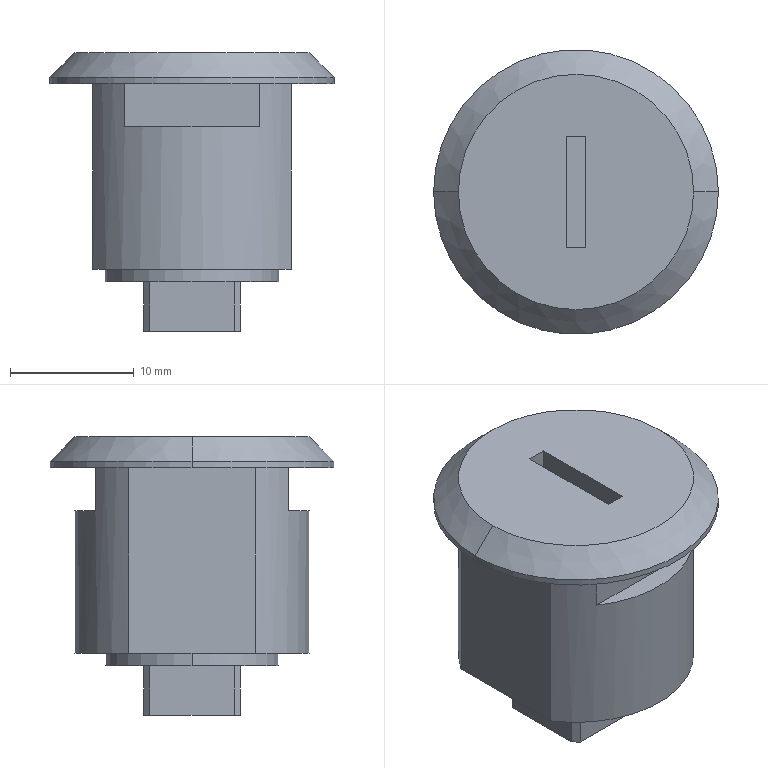Part | SolidWorks | features BaseBody 1 | 1 solid | 35 faces | box 23 x 23 x 22.5 mm | volume 4876 mm3 | plane 25 | cylinder 8 | cone 2 | commonest cylinder face diameters 3.545 x2 14 x2 19 x2 23 x2
STEP:
#1=CARTESIAN_POINT('',(9.6,1003.,461.7));
#2=VERTEX_POINT('',#1);
#3=CARTESIAN_POINT('',(-9.4,1003.,461.7));
#4=VERTEX_POINT('',#3);
#5=CARTESIAN_POINT('',(0.1,1003.,461.7));
#6=DIRECTION('',(0.,0.,-1.));
#7=DIRECTION('',(1.,0.,0.));
#8=AXIS2_PLACEMENT_3D('',#5,#6,#7);
#9=CIRCLE('',#8,9.5);
#10=EDGE_CURVE('',#2,#4,#9,.T.);
#11=ORIENTED_EDGE('',*,*,#10,.T.);
#12=CARTESIAN_POINT('',(-11.4,1003.,459.7));
#13=VERTEX_POINT('',#12);
#14=CARTESIAN_POINT('',(-11.4,1003.,459.7));
#15=DIRECTION('',(-0.7071,0.,-0.7071));
#16=VECTOR('',#15,1000.);
#17=LINE('',#14,#16);
#18=EDGE_CURVE('',#4,#13,#17,.T.);
#19=ORIENTED_EDGE('',*,*,#18,.T.);
#20=CARTESIAN_POINT('',(11.6,1003.,459.7));
#21=VERTEX_POINT('',#20);
#22=CARTESIAN_POINT('',(0.1,1003.,459.7));
#23=DIRECTION('',(0.,0.,1.));
#24=DIRECTION('',(1.,0.,0.));
#25=AXIS2_PLACEMENT_3D('',#22,#23,#24);
#26=CIRCLE('',#25,11.5);
#27=EDGE_CURVE('',#13,#21,#26,.T.);
#28=ORIENTED_EDGE('',*,*,#27,.T.);
#29=CARTESIAN_POINT('',(11.6,1003.,459.7));
#30=DIRECTION('',(0.7071,0.,-0.7071));
#31=VECTOR('',#30,1000.);
#32=LINE('',#29,#31);
#33=EDGE_CURVE('',#2,#21,#32,.T.);
#34=ORIENTED_EDGE('',*,*,#33,.F.);
#35=EDGE_LOOP('',(#11,#19,#28,#34));
#36=FACE_OUTER_BOUND('',#35,.T.);
#37=CARTESIAN_POINT('',(0.1,1003.,459.7));
#38=DIRECTION('',(0.,0.,-1.));
#39=DIRECTION('',(1.,0.,0.));
#40=AXIS2_PLACEMENT_3D('',#37,#38,#39);
#41=CONICAL_SURFACE('',#40,11.5,0.7854);
#42=ADVANCED_FACE('',(#36),#41,.T.);
#43=ORIENTED_EDGE('',*,*,#27,.F.);
#44=CARTESIAN_POINT('',(-11.4,1003.,459.2));
#45=VERTEX_POINT('',#44);
#46=CARTESIAN_POINT('',(-11.4,1003.,459.2));
#47=DIRECTION('',(0.,0.,-1.));
#48=VECTOR('',#47,1000.);
#49=LINE('',#46,#48);
#50=EDGE_CURVE('',#13,#45,#49,.T.);
#51=ORIENTED_EDGE('',*,*,#50,.T.);
#52=CARTESIAN_POINT('',(11.6,1003.,459.2));
#53=VERTEX_POINT('',#52);
#54=CARTESIAN_POINT('',(0.1,1003.,459.2));
#55=DIRECTION('',(0.,0.,1.));
#56=DIRECTION('',(1.,0.,0.));
#57=AXIS2_PLACEMENT_3D('',#54,#55,#56);
#58=CIRCLE('',#57,11.5);
#59=EDGE_CURVE('',#45,#53,#58,.T.);
#60=ORIENTED_EDGE('',*,*,#59,.T.);
#61=CARTESIAN_POINT('',(11.6,1003.,459.2));
#62=DIRECTION('',(0.,0.,-1.));
#63=VECTOR('',#62,1000.);
#64=LINE('',#61,#63);
#65=EDGE_CURVE('',#21,#53,#64,.T.);
#66=ORIENTED_EDGE('',*,*,#65,.F.);
#67=EDGE_LOOP('',(#43,#51,#60,#66));
#68=FACE_OUTER_BOUND('',#67,.T.);
#69=CARTESIAN_POINT('',(0.1,1003.,459.2));
#70=DIRECTION('',(0.,0.,-1.));
#71=DIRECTION('',(1.,0.,0.));
#72=AXIS2_PLACEMENT_3D('',#69,#70,#71);
#73=CYLINDRICAL_SURFACE('',#72,11.5);
#74=ADVANCED_FACE('',(#68),#73,.T.);
#75=CARTESIAN_POINT('',(-6.9,1003.,443.2));
#76=VERTEX_POINT('',#75);
#77=CARTESIAN_POINT('',(7.1,1003.,443.2));
#78=VERTEX_POINT('',#77);
#79=CARTESIAN_POINT('',(0.1,1003.,443.2));
#80=DIRECTION('',(0.,0.,1.));
#81=DIRECTION('',(-1.,0.,0.));
#82=AXIS2_PLACEMENT_3D('',#79,#80,#81);
#83=CIRCLE('',#82,7.);
#84=EDGE_CURVE('',#76,#78,#83,.T.);
#85=ORIENTED_EDGE('',*,*,#84,.T.);
#86=CARTESIAN_POINT('',(7.1,1003.,444.2));
#87=VERTEX_POINT('',#86);
#88=CARTESIAN_POINT('',(7.1,1003.,444.2));
#89=DIRECTION('',(0.,0.,1.));
#90=VECTOR('',#89,1000.);
#91=LINE('',#88,#90);
#92=EDGE_CURVE('',#78,#87,#91,.T.);
#93=ORIENTED_EDGE('',*,*,#92,.T.);
#94=CARTESIAN_POINT('',(-6.9,1003.,444.2));
#95=VERTEX_POINT('',#94);
#96=CARTESIAN_POINT('',(0.1,1003.,444.2));
#97=DIRECTION('',(0.,0.,1.));
#98=DIRECTION('',(-1.,0.,0.));
#99=AXIS2_PLACEMENT_3D('',#96,#97,#98);
#100=CIRCLE('',#99,7.);
#101=EDGE_CURVE('',#95,#87,#100,.T.);
#102=ORIENTED_EDGE('',*,*,#101,.F.);
#103=CARTESIAN_POINT('',(-6.9,1003.,444.2));
#104=DIRECTION('',(0.,0.,1.));
#105=VECTOR('',#104,1000.);
#106=LINE('',#103,#105);
#107=EDGE_CURVE('',#76,#95,#106,.T.);
#108=ORIENTED_EDGE('',*,*,#107,.F.);
#109=EDGE_LOOP('',(#85,#93,#102,#108));
#110=FACE_OUTER_BOUND('',#109,.T.);
#111=CARTESIAN_POINT('',(0.1,1003.,444.2));
#112=DIRECTION('',(0.,0.,1.));
#113=DIRECTION('',(-1.,0.,0.));
#114=AXIS2_PLACEMENT_3D('',#111,#112,#113);
#115=CYLINDRICAL_SURFACE('',#114,7.);
#116=ADVANCED_FACE('',(#110),#115,.T.);
#117=CARTESIAN_POINT('',(-1.673,1003.,445.2));
#118=VERTEX_POINT('',#117);
#119=CARTESIAN_POINT('',(1.872,1003.,445.2));
#120=VERTEX_POINT('',#119);
#121=CARTESIAN_POINT('',(0.1,1003.,445.2));
#122=DIRECTION('',(0.,0.,-1.));
#123=DIRECTION('',(1.,0.,0.));
#124=AXIS2_PLACEMENT_3D('',#121,#122,#123);
#125=CIRCLE('',#124,1.773);
#126=EDGE_CURVE('',#118,#120,#125,.T.);
#127=ORIENTED_EDGE('',*,*,#126,.F.);
#128=CARTESIAN_POINT('',(-1.673,1003.,439.2));
#129=VERTEX_POINT('',#128);
#130=CARTESIAN_POINT('',(-1.673,1003.,439.2));
#131=DIRECTION('',(0.,0.,-1.));
#132=VECTOR('',#131,1000.);
#133=LINE('',#130,#132);
#134=EDGE_CURVE('',#118,#129,#133,.T.);
#135=ORIENTED_EDGE('',*,*,#134,.T.);
#136=CARTESIAN_POINT('',(1.872,1003.,439.2));
#137=VERTEX_POINT('',#136);
#138=CARTESIAN_POINT('',(0.1,1003.,439.2));
#139=DIRECTION('',(0.,0.,-1.));
#140=DIRECTION('',(1.,0.,0.));
#141=AXIS2_PLACEMENT_3D('',#138,#139,#140);
#142=CIRCLE('',#141,1.772);
#143=EDGE_CURVE('',#129,#137,#142,.T.);
#144=ORIENTED_EDGE('',*,*,#143,.T.);
#145=CARTESIAN_POINT('',(1.872,1003.,439.2));
#146=DIRECTION('',(0.,0.,-1.));
#147=VECTOR('',#146,1000.);
#148=LINE('',#145,#147);
#149=EDGE_CURVE('',#120,#137,#148,.T.);
#150=ORIENTED_EDGE('',*,*,#149,.F.);
#151=EDGE_LOOP('',(#127,#135,#144,#150));
#152=FACE_OUTER_BOUND('',#151,.T.);
#153=CARTESIAN_POINT('',(0.1,1003.,439.2));
#154=DIRECTION('',(0.,0.,-1.));
#155=DIRECTION('',(1.,0.,0.));
#156=AXIS2_PLACEMENT_3D('',#153,#154,#155);
#157=CYLINDRICAL_SURFACE('',#156,1.772);
#158=ADVANCED_FACE('',(#152),#157,.F.);
#159=ORIENTED_EDGE('',*,*,#10,.F.);
#160=CARTESIAN_POINT('',(0.1,1003.,461.7));
#161=DIRECTION('',(0.,0.,-1.));
#162=DIRECTION('',(1.,0.,0.));
#163=AXIS2_PLACEMENT_3D('',#160,#161,#162);
#164=CIRCLE('',#163,9.5);
#165=EDGE_CURVE('',#4,#2,#164,.T.);
#166=ORIENTED_EDGE('',*,*,#165,.F.);
#167=EDGE_LOOP('',(#159,#166));
#168=FACE_OUTER_BOUND('',#167,.T.);
#169=CARTESIAN_POINT('',(-0.7,1007.5,461.7));
#170=VERTEX_POINT('',#169);
#171=CARTESIAN_POINT('',(-0.7,998.5,461.7));
#172=VERTEX_POINT('',#171);
#173=CARTESIAN_POINT('',(-0.7,1003.,461.7));
#174=DIRECTION('',(0.,-1.,0.));
#175=VECTOR('',#174,1000.);
#176=LINE('',#173,#175);
#177=EDGE_CURVE('',#170,#172,#176,.T.);
#178=ORIENTED_EDGE('',*,*,#177,.F.);
#179=CARTESIAN_POINT('',(0.9,1007.5,461.7));
#180=VERTEX_POINT('',#179);
#181=CARTESIAN_POINT('',(0.9,1007.5,461.7));
#182=DIRECTION('',(1.,0.,0.));
#183=VECTOR('',#182,1000.);
#184=LINE('',#181,#183);
#185=EDGE_CURVE('',#170,#180,#184,.T.);
#186=ORIENTED_EDGE('',*,*,#185,.T.);
#187=CARTESIAN_POINT('',(0.9,998.5,461.7));
#188=VERTEX_POINT('',#187);
#189=CARTESIAN_POINT('',(0.9,1003.,461.7));
#190=DIRECTION('',(0.,1.,0.));
#191=VECTOR('',#190,1000.);
#192=LINE('',#189,#191);
#193=EDGE_CURVE('',#188,#180,#192,.T.);
#194=ORIENTED_EDGE('',*,*,#193,.F.);
#195=CARTESIAN_POINT('',(-0.7,998.5,461.7));
#196=DIRECTION('',(-1.,0.,0.));
#197=VECTOR('',#196,1000.);
#198=LINE('',#195,#197);
#199=EDGE_CURVE('',#188,#172,#198,.T.);
#200=ORIENTED_EDGE('',*,*,#199,.T.);
#201=EDGE_LOOP('',(#178,#186,#194,#200));
#202=FACE_BOUND('',#201,.T.);
#203=CARTESIAN_POINT('',(0.1,1003.,461.7));
#204=DIRECTION('',(0.,0.,-1.));
#205=DIRECTION('',(1.,0.,0.));
#206=AXIS2_PLACEMENT_3D('',#203,#204,#205);
#207=PLANE('',#206);
#208=ADVANCED_FACE('',(#168,#202),#207,.F.);
#209=ORIENTED_EDGE('',*,*,#18,.F.);
#210=ORIENTED_EDGE('',*,*,#165,.T.);
#211=ORIENTED_EDGE('',*,*,#33,.T.);
#212=CARTESIAN_POINT('',(0.1,1003.,459.7));
#213=DIRECTION('',(0.,0.,1.));
#214=DIRECTION('',(1.,0.,0.));
#215=AXIS2_PLACEMENT_3D('',#212,#213,#214);
#216=CIRCLE('',#215,11.5);
#217=EDGE_CURVE('',#21,#13,#216,.T.);
#218=ORIENTED_EDGE('',*,*,#217,.T.);
#219=EDGE_LOOP('',(#209,#210,#211,#218));
#220=FACE_OUTER_BOUND('',#219,.T.);
#221=CARTESIAN_POINT('',(0.1,1003.,459.7));
#222=DIRECTION('',(0.,0.,-1.));
#223=DIRECTION('',(1.,0.,0.));
#224=AXIS2_PLACEMENT_3D('',#221,#222,#223);
#225=CONICAL_SURFACE('',#224,11.5,0.7854);
#226=ADVANCED_FACE('',(#220),#225,.T.);
#227=CARTESIAN_POINT('',(-0.7,998.5,446.74));
#228=VERTEX_POINT('',#227);
#229=CARTESIAN_POINT('',(-0.7,998.5,446.74));
#230=DIRECTION('',(0.,0.,1.));
#231=VECTOR('',#230,1000.);
#232=LINE('',#229,#231);
#233=EDGE_CURVE('',#228,#172,#232,.T.);
#234=ORIENTED_EDGE('',*,*,#233,.F.);
#235=CARTESIAN_POINT('',(-0.7,1007.5,446.74));
#236=VERTEX_POINT('',#235);
#237=CARTESIAN_POINT('',(-0.7,1007.5,446.74));
#238=DIRECTION('',(0.,-1.,0.));
#239=VECTOR('',#238,1000.);
#240=LINE('',#237,#239);
#241=EDGE_CURVE('',#236,#228,#240,.T.);
#242=ORIENTED_EDGE('',*,*,#241,.F.);
#243=CARTESIAN_POINT('',(-0.7,1007.5,446.74));
#244=DIRECTION('',(0.,0.,-1.));
#245=VECTOR('',#244,1000.);
#246=LINE('',#243,#245);
#247=EDGE_CURVE('',#170,#236,#246,.T.);
#248=ORIENTED_EDGE('',*,*,#247,.F.);
#249=ORIENTED_EDGE('',*,*,#177,.T.);
#250=EDGE_LOOP('',(#234,#242,#248,#249));
#251=FACE_OUTER_BOUND('',#250,.T.);
#252=CARTESIAN_POINT('',(-0.7,1007.5,446.74));
#253=DIRECTION('',(-1.,0.,0.));
#254=DIRECTION('',(0.,1.,0.));
#255=AXIS2_PLACEMENT_3D('',#252,#253,#254);
#256=PLANE('',#255);
#257=ADVANCED_FACE('',(#251),#256,.F.);
#258=CARTESIAN_POINT('',(0.9,1007.5,446.74));
#259=VERTEX_POINT('',#258);
#260=CARTESIAN_POINT('',(0.9,1007.5,446.74));
#261=DIRECTION('',(0.,0.,1.));
#262=VECTOR('',#261,1000.);
#263=LINE('',#260,#262);
#264=EDGE_CURVE('',#259,#180,#263,.T.);
#265=ORIENTED_EDGE('',*,*,#264,.F.);
#266=CARTESIAN_POINT('',(0.9,998.5,446.74));
#267=VERTEX_POINT('',#266);
#268=CARTESIAN_POINT('',(0.9,998.5,446.74));
#269=DIRECTION('',(0.,1.,0.));
#270=VECTOR('',#269,1000.);
#271=LINE('',#268,#270);
#272=EDGE_CURVE('',#267,#259,#271,.T.);
#273=ORIENTED_EDGE('',*,*,#272,.F.);
#274=CARTESIAN_POINT('',(0.9,998.5,446.74));
#275=DIRECTION('',(0.,0.,-1.));
#276=VECTOR('',#275,1000.);
#277=LINE('',#274,#276);
#278=EDGE_CURVE('',#188,#267,#277,.T.);
#279=ORIENTED_EDGE('',*,*,#278,.F.);
#280=ORIENTED_EDGE('',*,*,#193,.T.);
#281=EDGE_LOOP('',(#265,#273,#279,#280));
#282=FACE_OUTER_BOUND('',#281,.T.);
#283=CARTESIAN_POINT('',(0.9,998.5,446.74));
#284=DIRECTION('',(1.,0.,0.));
#285=DIRECTION('',(0.,-1.,0.));
#286=AXIS2_PLACEMENT_3D('',#283,#284,#285);
#287=PLANE('',#286);
#288=ADVANCED_FACE('',(#282),#287,.F.);
#289=ORIENTED_EDGE('',*,*,#50,.F.);
#290=ORIENTED_EDGE('',*,*,#217,.F.);
#291=ORIENTED_EDGE('',*,*,#65,.T.);
#292=CARTESIAN_POINT('',(0.1,1003.,459.2));
#293=DIRECTION('',(0.,0.,1.));
#294=DIRECTION('',(1.,0.,0.));
#295=AXIS2_PLACEMENT_3D('',#292,#293,#294);
#296=CIRCLE('',#295,11.5);
#297=EDGE_CURVE('',#53,#45,#296,.T.);
#298=ORIENTED_EDGE('',*,*,#297,.T.);
#299=EDGE_LOOP('',(#289,#290,#291,#298));
#300=FACE_OUTER_BOUND('',#299,.T.);
#301=CARTESIAN_POINT('',(0.1,1003.,459.2));
#302=DIRECTION('',(0.,0.,-1.));
#303=DIRECTION('',(1.,0.,0.));
#304=AXIS2_PLACEMENT_3D('',#301,#302,#303);
#305=CYLINDRICAL_SURFACE('',#304,11.5);
#306=ADVANCED_FACE('',(#300),#305,.T.);
#307=ORIENTED_EDGE('',*,*,#278,.T.);
#308=CARTESIAN_POINT('',(-0.7,998.5,446.74));
#309=DIRECTION('',(1.,0.,0.));
#310=VECTOR('',#309,1000.);
#311=LINE('',#308,#310);
#312=EDGE_CURVE('',#228,#267,#311,.T.);
#313=ORIENTED_EDGE('',*,*,#312,.F.);
#314=ORIENTED_EDGE('',*,*,#233,.T.);
#315=ORIENTED_EDGE('',*,*,#199,.F.);
#316=EDGE_LOOP('',(#307,#313,#314,#315));
#317=FACE_OUTER_BOUND('',#316,.T.);
#318=CARTESIAN_POINT('',(-0.7,998.5,446.74));
#319=DIRECTION('',(0.,-1.,0.));
#320=DIRECTION('',(-1.,0.,0.));
#321=AXIS2_PLACEMENT_3D('',#318,#319,#320);
#322=PLANE('',#321);
#323=ADVANCED_FACE('',(#317),#322,.F.);
#324=ORIENTED_EDGE('',*,*,#312,.T.);
#325=ORIENTED_EDGE('',*,*,#272,.T.);
#326=CARTESIAN_POINT('',(-0.7,1007.5,446.74));
#327=DIRECTION('',(1.,0.,0.));
#328=VECTOR('',#327,1000.);
#329=LINE('',#326,#328);
#330=EDGE_CURVE('',#236,#259,#329,.T.);
#331=ORIENTED_EDGE('',*,*,#330,.F.);
#332=ORIENTED_EDGE('',*,*,#241,.T.);
#333=EDGE_LOOP('',(#324,#325,#331,#332));
#334=FACE_OUTER_BOUND('',#333,.T.);
#335=CARTESIAN_POINT('',(-0.7,1007.5,446.74));
#336=DIRECTION('',(0.,0.,-1.));
#337=DIRECTION('',(1.,0.,0.));
#338=AXIS2_PLACEMENT_3D('',#335,#336,#337);
#339=PLANE('',#338);
#340=ADVANCED_FACE('',(#334),#339,.F.);
#341=ORIENTED_EDGE('',*,*,#247,.T.);
#342=ORIENTED_EDGE('',*,*,#330,.T.);
#343=ORIENTED_EDGE('',*,*,#264,.T.);
#344=ORIENTED_EDGE('',*,*,#185,.F.);
#345=EDGE_LOOP('',(#341,#342,#343,#344));
#346=FACE_OUTER_BOUND('',#345,.T.);
#347=CARTESIAN_POINT('',(0.9,1007.5,446.74));
#348=DIRECTION('',(0.,1.,0.));
#349=DIRECTION('',(1.,0.,0.));
#350=AXIS2_PLACEMENT_3D('',#347,#348,#349);
#351=PLANE('',#350);
#352=ADVANCED_FACE('',(#346),#351,.F.);
#353=ORIENTED_EDGE('',*,*,#297,.F.);
#354=ORIENTED_EDGE('',*,*,#59,.F.);
#355=EDGE_LOOP('',(#353,#354));
#356=FACE_OUTER_BOUND('',#355,.T.);
#357=CARTESIAN_POINT('',(-5.323,1010.8,459.2));
#358=VERTEX_POINT('',#357);
#359=CARTESIAN_POINT('',(-7.9,1008.123,459.2));
#360=VERTEX_POINT('',#359);
#361=CARTESIAN_POINT('',(0.1,1003.,459.2));
#362=DIRECTION('',(0.,0.,1.));
#363=DIRECTION('',(1.,0.,0.));
#364=AXIS2_PLACEMENT_3D('',#361,#362,#363);
#365=CIRCLE('',#364,9.5);
#366=EDGE_CURVE('',#358,#360,#365,.T.);
#367=ORIENTED_EDGE('',*,*,#366,.T.);
#368=CARTESIAN_POINT('',(-7.9,997.877,459.2));
#369=VERTEX_POINT('',#368);
#370=CARTESIAN_POINT('',(-7.9,1003.,459.2));
#371=DIRECTION('',(0.,-1.,0.));
#372=VECTOR('',#371,1000.);
#373=LINE('',#370,#372);
#374=EDGE_CURVE('',#360,#369,#373,.T.);
#375=ORIENTED_EDGE('',*,*,#374,.T.);
#376=CARTESIAN_POINT('',(-5.323,995.2,459.2));
#377=VERTEX_POINT('',#376);
#378=CARTESIAN_POINT('',(0.1,1003.,459.2));
#379=DIRECTION('',(0.,0.,1.));
#380=DIRECTION('',(1.,0.,0.));
#381=AXIS2_PLACEMENT_3D('',#378,#379,#380);
#382=CIRCLE('',#381,9.5);
#383=EDGE_CURVE('',#369,#377,#382,.T.);
#384=ORIENTED_EDGE('',*,*,#383,.T.);
#385=CARTESIAN_POINT('',(5.523,995.2,459.2));
#386=VERTEX_POINT('',#385);
#387=CARTESIAN_POINT('',(0.1,995.2,459.2));
#388=DIRECTION('',(1.,0.,0.));
#389=VECTOR('',#388,1000.);
#390=LINE('',#387,#389);
#391=EDGE_CURVE('',#377,#386,#390,.T.);
#392=ORIENTED_EDGE('',*,*,#391,.T.);
#393=CARTESIAN_POINT('',(8.1,997.877,459.2));
#394=VERTEX_POINT('',#393);
#395=CARTESIAN_POINT('',(0.1,1003.,459.2));
#396=DIRECTION('',(0.,0.,1.));
#397=DIRECTION('',(1.,0.,0.));
#398=AXIS2_PLACEMENT_3D('',#395,#396,#397);
#399=CIRCLE('',#398,9.5);
#400=EDGE_CURVE('',#386,#394,#399,.T.);
#401=ORIENTED_EDGE('',*,*,#400,.T.);
#402=CARTESIAN_POINT('',(8.1,1008.123,459.2));
#403=VERTEX_POINT('',#402);
#404=CARTESIAN_POINT('',(8.1,1003.,459.2));
#405=DIRECTION('',(0.,1.,0.));
#406=VECTOR('',#405,1000.);
#407=LINE('',#404,#406);
#408=EDGE_CURVE('',#394,#403,#407,.T.);
#409=ORIENTED_EDGE('',*,*,#408,.T.);
#410=CARTESIAN_POINT('',(5.523,1010.8,459.2));
#411=VERTEX_POINT('',#410);
#412=CARTESIAN_POINT('',(0.1,1003.,459.2));
#413=DIRECTION('',(0.,0.,1.));
#414=DIRECTION('',(1.,0.,0.));
#415=AXIS2_PLACEMENT_3D('',#412,#413,#414);
#416=CIRCLE('',#415,9.5);
#417=EDGE_CURVE('',#403,#411,#416,.T.);
#418=ORIENTED_EDGE('',*,*,#417,.T.);
#419=CARTESIAN_POINT('',(0.1,1010.8,459.2));
#420=DIRECTION('',(-1.,0.,0.));
#421=VECTOR('',#420,1000.);
#422=LINE('',#419,#421);
#423=EDGE_CURVE('',#411,#358,#422,.T.);
#424=ORIENTED_EDGE('',*,*,#423,.T.);
#425=EDGE_LOOP('',(#367,#375,#384,#392,#401,#409,#418,#424));
#426=FACE_BOUND('',#425,.T.);
#427=CARTESIAN_POINT('',(0.1,1003.,459.2));
#428=DIRECTION('',(0.,0.,-1.));
#429=DIRECTION('',(1.,0.,0.));
#430=AXIS2_PLACEMENT_3D('',#427,#428,#429);
#431=PLANE('',#430);
#432=ADVANCED_FACE('',(#356,#426),#431,.T.);
#433=CARTESIAN_POINT('',(-7.9,997.877,444.2));
#434=VERTEX_POINT('',#433);
#435=CARTESIAN_POINT('',(-7.9,997.877,459.2));
#436=DIRECTION('',(0.,0.,1.));
#437=VECTOR('',#436,1000.);
#438=LINE('',#435,#437);
#439=EDGE_CURVE('',#434,#369,#438,.T.);
#440=ORIENTED_EDGE('',*,*,#439,.T.);
#441=ORIENTED_EDGE('',*,*,#374,.F.);
#442=CARTESIAN_POINT('',(-7.9,1008.123,444.2));
#443=VERTEX_POINT('',#442);
#444=CARTESIAN_POINT('',(-7.9,1008.123,459.2));
#445=DIRECTION('',(0.,0.,-1.));
#446=VECTOR('',#445,1000.);
#447=LINE('',#444,#446);
#448=EDGE_CURVE('',#360,#443,#447,.T.);
#449=ORIENTED_EDGE('',*,*,#448,.T.);
#450=CARTESIAN_POINT('',(-7.9,908.38,444.2));
#451=DIRECTION('',(0.,-1.,0.));
#452=VECTOR('',#451,1000.);
#453=LINE('',#450,#452);
#454=EDGE_CURVE('',#443,#434,#453,.T.);
#455=ORIENTED_EDGE('',*,*,#454,.T.);
#456=EDGE_LOOP('',(#440,#441,#449,#455));
#457=FACE_OUTER_BOUND('',#456,.T.);
#458=CARTESIAN_POINT('',(-7.9,908.38,459.2));
#459=DIRECTION('',(-1.,0.,0.));
#460=DIRECTION('',(0.,1.,0.));
#461=AXIS2_PLACEMENT_3D('',#458,#459,#460);
#462=PLANE('',#461);
#463=ADVANCED_FACE('',(#457),#462,.T.);
#464=CARTESIAN_POINT('',(-5.323,1010.8,455.7));
#465=VERTEX_POINT('',#464);
#466=CARTESIAN_POINT('',(-5.323,1010.8,443.2));
#467=DIRECTION('',(0.,0.,-1.));
#468=VECTOR('',#467,1000.);
#469=LINE('',#466,#468);
#470=EDGE_CURVE('',#358,#465,#469,.T.);
#471=ORIENTED_EDGE('',*,*,#470,.T.);
#472=CARTESIAN_POINT('',(5.523,1010.8,455.7));
#473=VERTEX_POINT('',#472);
#474=CARTESIAN_POINT('',(0.1,1003.,455.7));
#475=DIRECTION('',(0.,0.,-1.));
#476=DIRECTION('',(1.,0.,0.));
#477=AXIS2_PLACEMENT_3D('',#474,#475,#476);
#478=CIRCLE('',#477,9.5);
#479=EDGE_CURVE('',#465,#473,#478,.T.);
#480=ORIENTED_EDGE('',*,*,#479,.T.);
#481=CARTESIAN_POINT('',(5.523,1010.8,443.2));
#482=DIRECTION('',(0.,0.,1.));
#483=VECTOR('',#482,1000.);
#484=LINE('',#481,#483);
#485=EDGE_CURVE('',#473,#411,#484,.T.);
#486=ORIENTED_EDGE('',*,*,#485,.T.);
#487=ORIENTED_EDGE('',*,*,#417,.F.);
#488=CARTESIAN_POINT('',(8.1,1008.123,444.2));
#489=VERTEX_POINT('',#488);
#490=CARTESIAN_POINT('',(8.1,1008.123,443.2));
#491=DIRECTION('',(0.,0.,-1.));
#492=VECTOR('',#491,1000.);
#493=LINE('',#490,#492);
#494=EDGE_CURVE('',#403,#489,#493,.T.);
#495=ORIENTED_EDGE('',*,*,#494,.T.);
#496=CARTESIAN_POINT('',(0.1,1003.,444.2));
#497=DIRECTION('',(0.,0.,1.));
#498=DIRECTION('',(1.,0.,0.));
#499=AXIS2_PLACEMENT_3D('',#496,#497,#498);
#500=CIRCLE('',#499,9.5);
#501=EDGE_CURVE('',#489,#443,#500,.T.);
#502=ORIENTED_EDGE('',*,*,#501,.T.);
#503=ORIENTED_EDGE('',*,*,#448,.F.);
#504=ORIENTED_EDGE('',*,*,#366,.F.);
#505=EDGE_LOOP('',(#471,#480,#486,#487,#495,#502,#503,#504));
#506=FACE_OUTER_BOUND('',#505,.T.);
#507=CARTESIAN_POINT('',(0.1,1003.,443.2));
#508=DIRECTION('',(0.,0.,-1.));
#509=DIRECTION('',(1.,0.,0.));
#510=AXIS2_PLACEMENT_3D('',#507,#508,#509);
#511=CYLINDRICAL_SURFACE('',#510,9.5);
#512=ADVANCED_FACE('',(#506),#511,.T.);
#513=CARTESIAN_POINT('',(83.61,1010.8,455.7));
#514=DIRECTION('',(1.,0.,0.));
#515=VECTOR('',#514,1000.);
#516=LINE('',#513,#515);
#517=EDGE_CURVE('',#465,#473,#516,.T.);
#518=ORIENTED_EDGE('',*,*,#517,.F.);
#519=ORIENTED_EDGE('',*,*,#470,.F.);
#520=ORIENTED_EDGE('',*,*,#423,.F.);
#521=ORIENTED_EDGE('',*,*,#485,.F.);
#522=EDGE_LOOP('',(#518,#519,#520,#521));
#523=FACE_OUTER_BOUND('',#522,.T.);
#524=CARTESIAN_POINT('',(83.61,1010.8,455.7));
#525=DIRECTION('',(0.,-1.,0.));
#526=DIRECTION('',(0.,0.,-1.));
#527=AXIS2_PLACEMENT_3D('',#524,#525,#526);
#528=PLANE('',#527);
#529=ADVANCED_FACE('',(#523),#528,.F.);
#530=ORIENTED_EDGE('',*,*,#494,.F.);
#531=ORIENTED_EDGE('',*,*,#408,.F.);
#532=CARTESIAN_POINT('',(8.1,997.877,444.2));
#533=VERTEX_POINT('',#532);
#534=CARTESIAN_POINT('',(8.1,997.877,459.2));
#535=DIRECTION('',(0.,0.,1.));
#536=VECTOR('',#535,1000.);
#537=LINE('',#534,#536);
#538=EDGE_CURVE('',#533,#394,#537,.T.);
#539=ORIENTED_EDGE('',*,*,#538,.F.);
#540=CARTESIAN_POINT('',(8.1,963.32,444.2));
#541=DIRECTION('',(0.,-1.,0.));
#542=VECTOR('',#541,1000.);
#543=LINE('',#540,#542);
#544=EDGE_CURVE('',#489,#533,#543,.T.);
#545=ORIENTED_EDGE('',*,*,#544,.F.);
#546=EDGE_LOOP('',(#530,#531,#539,#545));
#547=FACE_OUTER_BOUND('',#546,.T.);
#548=CARTESIAN_POINT('',(8.1,963.32,459.2));
#549=DIRECTION('',(-1.,0.,0.));
#550=DIRECTION('',(0.,0.,-1.));
#551=AXIS2_PLACEMENT_3D('',#548,#549,#550);
#552=PLANE('',#551);
#553=ADVANCED_FACE('',(#547),#552,.F.);
#554=CARTESIAN_POINT('',(5.523,995.2,455.7));
#555=VERTEX_POINT('',#554);
#556=CARTESIAN_POINT('',(5.523,995.2,443.2));
#557=DIRECTION('',(0.,0.,-1.));
#558=VECTOR('',#557,1000.);
#559=LINE('',#556,#558);
#560=EDGE_CURVE('',#386,#555,#559,.T.);
#561=ORIENTED_EDGE('',*,*,#560,.T.);
#562=CARTESIAN_POINT('',(-5.323,995.2,455.7));
#563=VERTEX_POINT('',#562);
#564=CARTESIAN_POINT('',(0.1,1003.,455.7));
#565=DIRECTION('',(0.,0.,-1.));
#566=DIRECTION('',(1.,0.,0.));
#567=AXIS2_PLACEMENT_3D('',#564,#565,#566);
#568=CIRCLE('',#567,9.5);
#569=EDGE_CURVE('',#555,#563,#568,.T.);
#570=ORIENTED_EDGE('',*,*,#569,.T.);
#571=CARTESIAN_POINT('',(-5.323,995.2,443.2));
#572=DIRECTION('',(0.,0.,1.));
#573=VECTOR('',#572,1000.);
#574=LINE('',#571,#573);
#575=EDGE_CURVE('',#563,#377,#574,.T.);
#576=ORIENTED_EDGE('',*,*,#575,.T.);
#577=ORIENTED_EDGE('',*,*,#383,.F.);
#578=ORIENTED_EDGE('',*,*,#439,.F.);
#579=CARTESIAN_POINT('',(0.1,1003.,444.2));
#580=DIRECTION('',(0.,0.,1.));
#581=DIRECTION('',(1.,0.,0.));
#582=AXIS2_PLACEMENT_3D('',#579,#580,#581);
#583=CIRCLE('',#582,9.5);
#584=EDGE_CURVE('',#434,#533,#583,.T.);
#585=ORIENTED_EDGE('',*,*,#584,.T.);
#586=ORIENTED_EDGE('',*,*,#538,.T.);
#587=ORIENTED_EDGE('',*,*,#400,.F.);
#588=EDGE_LOOP('',(#561,#570,#576,#577,#578,#585,#586,#587));
#589=FACE_OUTER_BOUND('',#588,.T.);
#590=CARTESIAN_POINT('',(0.1,1003.,443.2));
#591=DIRECTION('',(0.,0.,-1.));
#592=DIRECTION('',(1.,0.,0.));
#593=AXIS2_PLACEMENT_3D('',#590,#591,#592);
#594=CYLINDRICAL_SURFACE('',#593,9.5);
#595=ADVANCED_FACE('',(#589),#594,.T.);
#596=CARTESIAN_POINT('',(83.61,995.2,455.7));
#597=DIRECTION('',(-1.,0.,0.));
#598=VECTOR('',#597,1000.);
#599=LINE('',#596,#598);
#600=EDGE_CURVE('',#555,#563,#599,.T.);
#601=ORIENTED_EDGE('',*,*,#600,.F.);
#602=ORIENTED_EDGE('',*,*,#560,.F.);
#603=ORIENTED_EDGE('',*,*,#391,.F.);
#604=ORIENTED_EDGE('',*,*,#575,.F.);
#605=EDGE_LOOP('',(#601,#602,#603,#604));
#606=FACE_OUTER_BOUND('',#605,.T.);
#607=CARTESIAN_POINT('',(83.61,995.2,455.7));
#608=DIRECTION('',(0.,1.,0.));
#609=DIRECTION('',(0.,0.,1.));
#610=AXIS2_PLACEMENT_3D('',#607,#608,#609);
#611=PLANE('',#610);
#612=ADVANCED_FACE('',(#606),#611,.F.);
#613=ORIENTED_EDGE('',*,*,#454,.F.);
#614=ORIENTED_EDGE('',*,*,#501,.F.);
#615=ORIENTED_EDGE('',*,*,#544,.T.);
#616=ORIENTED_EDGE('',*,*,#584,.F.);
#617=EDGE_LOOP('',(#613,#614,#615,#616));
#618=FACE_OUTER_BOUND('',#617,.T.);
#619=ORIENTED_EDGE('',*,*,#101,.T.);
#620=CARTESIAN_POINT('',(0.1,1003.,444.2));
#621=DIRECTION('',(0.,0.,1.));
#622=DIRECTION('',(-1.,0.,0.));
#623=AXIS2_PLACEMENT_3D('',#620,#621,#622);
#624=CIRCLE('',#623,7.);
#625=EDGE_CURVE('',#87,#95,#624,.T.);
#626=ORIENTED_EDGE('',*,*,#625,.T.);
#627=EDGE_LOOP('',(#619,#626));
#628=FACE_BOUND('',#627,.T.);
#629=CARTESIAN_POINT('',(0.1075,1006.489,444.2));
#630=DIRECTION('',(0.,0.,-1.));
#631=DIRECTION('',(1.,0.,0.));
#632=AXIS2_PLACEMENT_3D('',#629,#630,#631);
#633=PLANE('',#632);
#634=ADVANCED_FACE('',(#618,#628),#633,.T.);
#635=ORIENTED_EDGE('',*,*,#479,.F.);
#636=ORIENTED_EDGE('',*,*,#517,.T.);
#637=EDGE_LOOP('',(#635,#636));
#638=FACE_OUTER_BOUND('',#637,.T.);
#639=CARTESIAN_POINT('',(83.61,1012.5,455.7));
#640=DIRECTION('',(0.,0.,-1.));
#641=DIRECTION('',(1.,0.,0.));
#642=AXIS2_PLACEMENT_3D('',#639,#640,#641);
#643=PLANE('',#642);
#644=ADVANCED_FACE('',(#638),#643,.F.);
#645=ORIENTED_EDGE('',*,*,#569,.F.);
#646=ORIENTED_EDGE('',*,*,#600,.T.);
#647=EDGE_LOOP('',(#645,#646));
#648=FACE_OUTER_BOUND('',#647,.T.);
#649=CARTESIAN_POINT('',(83.61,993.5,455.7));
#650=DIRECTION('',(0.,0.,-1.));
#651=DIRECTION('',(1.,0.,0.));
#652=AXIS2_PLACEMENT_3D('',#649,#650,#651);
#653=PLANE('',#652);
#654=ADVANCED_FACE('',(#648),#653,.F.);
#655=ORIENTED_EDGE('',*,*,#92,.F.);
#656=CARTESIAN_POINT('',(0.1,1003.,443.2));
#657=DIRECTION('',(0.,0.,1.));
#658=DIRECTION('',(-1.,0.,0.));
#659=AXIS2_PLACEMENT_3D('',#656,#657,#658);
#660=CIRCLE('',#659,7.);
#661=EDGE_CURVE('',#78,#76,#660,.T.);
#662=ORIENTED_EDGE('',*,*,#661,.T.);
#663=ORIENTED_EDGE('',*,*,#107,.T.);
#664=ORIENTED_EDGE('',*,*,#625,.F.);
#665=EDGE_LOOP('',(#655,#662,#663,#664));
#666=FACE_OUTER_BOUND('',#665,.T.);
#667=CARTESIAN_POINT('',(0.1,1003.,444.2));
#668=DIRECTION('',(0.,0.,1.));
#669=DIRECTION('',(-1.,0.,0.));
#670=AXIS2_PLACEMENT_3D('',#667,#668,#669);
#671=CYLINDRICAL_SURFACE('',#670,7.);
#672=ADVANCED_FACE('',(#666),#671,.T.);
#673=CARTESIAN_POINT('',(4.,1006.4,443.2));
#674=VERTEX_POINT('',#673);
#675=CARTESIAN_POINT('',(3.5,1006.9,443.2));
#676=VERTEX_POINT('',#675);
#677=CARTESIAN_POINT('',(4.,1006.4,443.2));
#678=DIRECTION('',(-0.7071,0.7071,0.));
#679=VECTOR('',#678,1000.);
#680=LINE('',#677,#679);
#681=EDGE_CURVE('',#674,#676,#680,.T.);
#682=ORIENTED_EDGE('',*,*,#681,.T.);
#683=CARTESIAN_POINT('',(-3.3,1006.9,443.2));
#684=VERTEX_POINT('',#683);
#685=CARTESIAN_POINT('',(0.1,1006.9,443.2));
#686=DIRECTION('',(1.,0.,0.));
#687=VECTOR('',#686,1000.);
#688=LINE('',#685,#687);
#689=EDGE_CURVE('',#684,#676,#688,.T.);
#690=ORIENTED_EDGE('',*,*,#689,.F.);
#691=CARTESIAN_POINT('',(-3.8,1006.4,443.2));
#692=VERTEX_POINT('',#691);
#693=CARTESIAN_POINT('',(-3.3,1006.9,443.2));
#694=DIRECTION('',(-0.7071,-0.7071,0.));
#695=VECTOR('',#694,1000.);
#696=LINE('',#693,#695);
#697=EDGE_CURVE('',#684,#692,#696,.T.);
#698=ORIENTED_EDGE('',*,*,#697,.T.);
#699=CARTESIAN_POINT('',(-3.8,999.6,443.2));
#700=VERTEX_POINT('',#699);
#701=CARTESIAN_POINT('',(-3.8,1003.,443.2));
#702=DIRECTION('',(0.,1.,0.));
#703=VECTOR('',#702,1000.);
#704=LINE('',#701,#703);
#705=EDGE_CURVE('',#700,#692,#704,.T.);
#706=ORIENTED_EDGE('',*,*,#705,.F.);
#707=CARTESIAN_POINT('',(-3.3,999.1,443.2));
#708=VERTEX_POINT('',#707);
#709=CARTESIAN_POINT('',(-3.8,999.6,443.2));
#710=DIRECTION('',(0.7071,-0.7071,0.));
#711=VECTOR('',#710,1000.);
#712=LINE('',#709,#711);
#713=EDGE_CURVE('',#700,#708,#712,.T.);
#714=ORIENTED_EDGE('',*,*,#713,.T.);
#715=CARTESIAN_POINT('',(3.5,999.1,443.2));
#716=VERTEX_POINT('',#715);
#717=CARTESIAN_POINT('',(0.1,999.1,443.2));
#718=DIRECTION('',(-1.,0.,0.));
#719=VECTOR('',#718,1000.);
#720=LINE('',#717,#719);
#721=EDGE_CURVE('',#716,#708,#720,.T.);
#722=ORIENTED_EDGE('',*,*,#721,.F.);
#723=CARTESIAN_POINT('',(4.,999.6,443.2));
#724=VERTEX_POINT('',#723);
#725=CARTESIAN_POINT('',(3.5,999.1,443.2));
#726=DIRECTION('',(0.7071,0.7071,0.));
#727=VECTOR('',#726,1000.);
#728=LINE('',#725,#727);
#729=EDGE_CURVE('',#716,#724,#728,.T.);
#730=ORIENTED_EDGE('',*,*,#729,.T.);
#731=CARTESIAN_POINT('',(4.,1003.,443.2));
#732=DIRECTION('',(0.,-1.,0.));
#733=VECTOR('',#732,1000.);
#734=LINE('',#731,#733);
#735=EDGE_CURVE('',#674,#724,#734,.T.);
#736=ORIENTED_EDGE('',*,*,#735,.F.);
#737=EDGE_LOOP('',(#682,#690,#698,#706,#714,#722,#730,#736));
#738=FACE_BOUND('',#737,.T.);
#739=ORIENTED_EDGE('',*,*,#84,.F.);
#740=ORIENTED_EDGE('',*,*,#661,.F.);
#741=EDGE_LOOP('',(#739,#740));
#742=FACE_OUTER_BOUND('',#741,.T.);
#743=CARTESIAN_POINT('',(0.1,1003.,443.2));
#744=DIRECTION('',(0.,0.,1.));
#745=DIRECTION('',(-1.,0.,0.));
#746=AXIS2_PLACEMENT_3D('',#743,#744,#745);
#747=PLANE('',#746);
#748=ADVANCED_FACE('',(#738,#742),#747,.F.);
#749=CARTESIAN_POINT('',(4.,999.6,439.2));
#750=VERTEX_POINT('',#749);
#751=CARTESIAN_POINT('',(4.,999.6,439.2));
#752=DIRECTION('',(0.,0.,1.));
#753=VECTOR('',#752,1000.);
#754=LINE('',#751,#753);
#755=EDGE_CURVE('',#750,#724,#754,.T.);
#756=ORIENTED_EDGE('',*,*,#755,.F.);
#757=CARTESIAN_POINT('',(4.,1006.4,439.2));
#758=VERTEX_POINT('',#757);
#759=CARTESIAN_POINT('',(4.,1006.9,439.2));
#760=DIRECTION('',(0.,-1.,0.));
#761=VECTOR('',#760,1000.);
#762=LINE('',#759,#761);
#763=EDGE_CURVE('',#758,#750,#762,.T.);
#764=ORIENTED_EDGE('',*,*,#763,.F.);
#765=CARTESIAN_POINT('',(4.,1006.4,439.2));
#766=DIRECTION('',(0.,0.,-1.));
#767=VECTOR('',#766,1000.);
#768=LINE('',#765,#767);
#769=EDGE_CURVE('',#674,#758,#768,.T.);
#770=ORIENTED_EDGE('',*,*,#769,.F.);
#771=ORIENTED_EDGE('',*,*,#735,.T.);
#772=EDGE_LOOP('',(#756,#764,#770,#771));
#773=FACE_OUTER_BOUND('',#772,.T.);
#774=CARTESIAN_POINT('',(4.,1006.9,439.2));
#775=DIRECTION('',(-1.,0.,0.));
#776=DIRECTION('',(0.,1.,0.));
#777=AXIS2_PLACEMENT_3D('',#774,#775,#776);
#778=PLANE('',#777);
#779=ADVANCED_FACE('',(#773),#778,.F.);
#780=CARTESIAN_POINT('',(-3.3,1006.9,439.2));
#781=VERTEX_POINT('',#780);
#782=CARTESIAN_POINT('',(-3.3,1006.9,439.2));
#783=DIRECTION('',(0.,0.,-1.));
#784=VECTOR('',#783,1000.);
#785=LINE('',#782,#784);
#786=EDGE_CURVE('',#684,#781,#785,.T.);
#787=ORIENTED_EDGE('',*,*,#786,.F.);
#788=ORIENTED_EDGE('',*,*,#689,.T.);
#789=CARTESIAN_POINT('',(3.5,1006.9,439.2));
#790=VERTEX_POINT('',#789);
#791=CARTESIAN_POINT('',(3.5,1006.9,439.2));
#792=DIRECTION('',(0.,0.,1.));
#793=VECTOR('',#792,1000.);
#794=LINE('',#791,#793);
#795=EDGE_CURVE('',#790,#676,#794,.T.);
#796=ORIENTED_EDGE('',*,*,#795,.F.);
#797=CARTESIAN_POINT('',(-3.8,1006.9,439.2));
#798=DIRECTION('',(1.,0.,0.));
#799=VECTOR('',#798,1000.);
#800=LINE('',#797,#799);
#801=EDGE_CURVE('',#781,#790,#800,.T.);
#802=ORIENTED_EDGE('',*,*,#801,.F.);
#803=EDGE_LOOP('',(#787,#788,#796,#802));
#804=FACE_OUTER_BOUND('',#803,.T.);
#805=CARTESIAN_POINT('',(-3.8,1006.9,439.2));
#806=DIRECTION('',(0.,-1.,0.));
#807=DIRECTION('',(-1.,0.,0.));
#808=AXIS2_PLACEMENT_3D('',#805,#806,#807);
#809=PLANE('',#808);
#810=ADVANCED_FACE('',(#804),#809,.F.);
#811=CARTESIAN_POINT('',(-3.8,999.6,439.2));
#812=VERTEX_POINT('',#811);
#813=CARTESIAN_POINT('',(-3.8,999.6,439.2));
#814=DIRECTION('',(0.,0.,-1.));
#815=VECTOR('',#814,1000.);
#816=LINE('',#813,#815);
#817=EDGE_CURVE('',#700,#812,#816,.T.);
#818=ORIENTED_EDGE('',*,*,#817,.F.);
#819=ORIENTED_EDGE('',*,*,#705,.T.);
#820=CARTESIAN_POINT('',(-3.8,1006.4,439.2));
#821=VERTEX_POINT('',#820);
#822=CARTESIAN_POINT('',(-3.8,1006.4,439.2));
#823=DIRECTION('',(0.,0.,1.));
#824=VECTOR('',#823,1000.);
#825=LINE('',#822,#824);
#826=EDGE_CURVE('',#821,#692,#825,.T.);
#827=ORIENTED_EDGE('',*,*,#826,.F.);
#828=CARTESIAN_POINT('',(-3.8,999.1,439.2));
#829=DIRECTION('',(0.,1.,0.));
#830=VECTOR('',#829,1000.);
#831=LINE('',#828,#830);
#832=EDGE_CURVE('',#812,#821,#831,.T.);
#833=ORIENTED_EDGE('',*,*,#832,.F.);
#834=EDGE_LOOP('',(#818,#819,#827,#833));
#835=FACE_OUTER_BOUND('',#834,.T.);
#836=CARTESIAN_POINT('',(-3.8,999.1,439.2));
#837=DIRECTION('',(1.,0.,0.));
#838=DIRECTION('',(0.,-1.,0.));
#839=AXIS2_PLACEMENT_3D('',#836,#837,#838);
#840=PLANE('',#839);
#841=ADVANCED_FACE('',(#835),#840,.F.);
#842=CARTESIAN_POINT('',(-3.3,999.1,439.2));
#843=VERTEX_POINT('',#842);
#844=CARTESIAN_POINT('',(-3.3,999.1,439.2));
#845=DIRECTION('',(0.,0.,1.));
#846=VECTOR('',#845,1000.);
#847=LINE('',#844,#846);
#848=EDGE_CURVE('',#843,#708,#847,.T.);
#849=ORIENTED_EDGE('',*,*,#848,.F.);
#850=CARTESIAN_POINT('',(3.5,999.1,439.2));
#851=VERTEX_POINT('',#850);
#852=CARTESIAN_POINT('',(4.,999.1,439.2));
#853=DIRECTION('',(-1.,0.,0.));
#854=VECTOR('',#853,1000.);
#855=LINE('',#852,#854);
#856=EDGE_CURVE('',#851,#843,#855,.T.);
#857=ORIENTED_EDGE('',*,*,#856,.F.);
#858=CARTESIAN_POINT('',(3.5,999.1,439.2));
#859=DIRECTION('',(0.,0.,-1.));
#860=VECTOR('',#859,1000.);
#861=LINE('',#858,#860);
#862=EDGE_CURVE('',#716,#851,#861,.T.);
#863=ORIENTED_EDGE('',*,*,#862,.F.);
#864=ORIENTED_EDGE('',*,*,#721,.T.);
#865=EDGE_LOOP('',(#849,#857,#863,#864));
#866=FACE_OUTER_BOUND('',#865,.T.);
#867=CARTESIAN_POINT('',(4.,999.1,439.2));
#868=DIRECTION('',(0.,1.,0.));
#869=DIRECTION('',(1.,0.,0.));
#870=AXIS2_PLACEMENT_3D('',#867,#868,#869);
#871=PLANE('',#870);
#872=ADVANCED_FACE('',(#866),#871,.F.);
#873=ORIENTED_EDGE('',*,*,#755,.T.);
#874=ORIENTED_EDGE('',*,*,#729,.F.);
#875=ORIENTED_EDGE('',*,*,#862,.T.);
#876=CARTESIAN_POINT('',(3.5,999.1,439.2));
#877=DIRECTION('',(-0.7071,-0.7071,0.));
#878=VECTOR('',#877,1000.);
#879=LINE('',#876,#878);
#880=EDGE_CURVE('',#750,#851,#879,.T.);
#881=ORIENTED_EDGE('',*,*,#880,.F.);
#882=EDGE_LOOP('',(#873,#874,#875,#881));
#883=FACE_OUTER_BOUND('',#882,.T.);
#884=CARTESIAN_POINT('',(3.5,999.1,439.2));
#885=DIRECTION('',(-0.7071,0.7071,0.));
#886=DIRECTION('',(0.7071,0.7071,0.));
#887=AXIS2_PLACEMENT_3D('',#884,#885,#886);
#888=PLANE('',#887);
#889=ADVANCED_FACE('',(#883),#888,.F.);
#890=CARTESIAN_POINT('',(-3.8,999.6,439.2));
#891=DIRECTION('',(0.7071,-0.7071,0.));
#892=VECTOR('',#891,1000.);
#893=LINE('',#890,#892);
#894=EDGE_CURVE('',#812,#843,#893,.T.);
#895=ORIENTED_EDGE('',*,*,#894,.F.);
#896=ORIENTED_EDGE('',*,*,#832,.T.);
#897=CARTESIAN_POINT('',(-3.3,1006.9,439.2));
#898=DIRECTION('',(-0.7071,-0.7071,0.));
#899=VECTOR('',#898,1000.);
#900=LINE('',#897,#899);
#901=EDGE_CURVE('',#781,#821,#900,.T.);
#902=ORIENTED_EDGE('',*,*,#901,.F.);
#903=ORIENTED_EDGE('',*,*,#801,.T.);
#904=CARTESIAN_POINT('',(4.,1006.4,439.2));
#905=DIRECTION('',(-0.7071,0.7071,0.));
#906=VECTOR('',#905,1000.);
#907=LINE('',#904,#906);
#908=EDGE_CURVE('',#758,#790,#907,.T.);
#909=ORIENTED_EDGE('',*,*,#908,.F.);
#910=ORIENTED_EDGE('',*,*,#763,.T.);
#911=ORIENTED_EDGE('',*,*,#880,.T.);
#912=ORIENTED_EDGE('',*,*,#856,.T.);
#913=EDGE_LOOP('',(#895,#896,#902,#903,#909,#910,#911,#912));
#914=FACE_OUTER_BOUND('',#913,.T.);
#915=CARTESIAN_POINT('',(0.1,1003.,439.2));
#916=DIRECTION('',(0.,0.,-1.));
#917=DIRECTION('',(1.,0.,0.));
#918=AXIS2_PLACEMENT_3D('',#915,#916,#917);
#919=CIRCLE('',#918,1.772);
#920=EDGE_CURVE('',#137,#129,#919,.T.);
#921=ORIENTED_EDGE('',*,*,#920,.F.);
#922=ORIENTED_EDGE('',*,*,#143,.F.);
#923=EDGE_LOOP('',(#921,#922));
#924=FACE_BOUND('',#923,.T.);
#925=CARTESIAN_POINT('',(4.,1006.9,439.2));
#926=DIRECTION('',(0.,0.,1.));
#927=DIRECTION('',(-1.,0.,0.));
#928=AXIS2_PLACEMENT_3D('',#925,#926,#927);
#929=PLANE('',#928);
#930=ADVANCED_FACE('',(#914,#924),#929,.F.);
#931=ORIENTED_EDGE('',*,*,#795,.T.);
#932=ORIENTED_EDGE('',*,*,#681,.F.);
#933=ORIENTED_EDGE('',*,*,#769,.T.);
#934=ORIENTED_EDGE('',*,*,#908,.T.);
#935=EDGE_LOOP('',(#931,#932,#933,#934));
#936=FACE_OUTER_BOUND('',#935,.T.);
#937=CARTESIAN_POINT('',(4.,1006.4,439.2));
#938=DIRECTION('',(-0.7071,-0.7071,0.));
#939=DIRECTION('',(-0.7071,0.7071,0.));
#940=AXIS2_PLACEMENT_3D('',#937,#938,#939);
#941=PLANE('',#940);
#942=ADVANCED_FACE('',(#936),#941,.F.);
#943=ORIENTED_EDGE('',*,*,#826,.T.);
#944=ORIENTED_EDGE('',*,*,#697,.F.);
#945=ORIENTED_EDGE('',*,*,#786,.T.);
#946=ORIENTED_EDGE('',*,*,#901,.T.);
#947=EDGE_LOOP('',(#943,#944,#945,#946));
#948=FACE_OUTER_BOUND('',#947,.T.);
#949=CARTESIAN_POINT('',(-3.3,1006.9,439.2));
#950=DIRECTION('',(0.7071,-0.7071,0.));
#951=DIRECTION('',(-0.7071,-0.7071,0.));
#952=AXIS2_PLACEMENT_3D('',#949,#950,#951);
#953=PLANE('',#952);
#954=ADVANCED_FACE('',(#948),#953,.F.);
#955=ORIENTED_EDGE('',*,*,#848,.T.);
#956=ORIENTED_EDGE('',*,*,#713,.F.);
#957=ORIENTED_EDGE('',*,*,#817,.T.);
#958=ORIENTED_EDGE('',*,*,#894,.T.);
#959=EDGE_LOOP('',(#955,#956,#957,#958));
#960=FACE_OUTER_BOUND('',#959,.T.);
#961=CARTESIAN_POINT('',(-3.8,999.6,439.2));
#962=DIRECTION('',(0.7071,0.7071,0.));
#963=DIRECTION('',(0.7071,-0.7071,0.));
#964=AXIS2_PLACEMENT_3D('',#961,#962,#963);
#965=PLANE('',#964);
#966=ADVANCED_FACE('',(#960),#965,.F.);
#967=ORIENTED_EDGE('',*,*,#134,.F.);
#968=CARTESIAN_POINT('',(0.1,1003.,445.2));
#969=DIRECTION('',(0.,0.,-1.));
#970=DIRECTION('',(1.,0.,0.));
#971=AXIS2_PLACEMENT_3D('',#968,#969,#970);
#972=CIRCLE('',#971,1.773);
#973=EDGE_CURVE('',#120,#118,#972,.T.);
#974=ORIENTED_EDGE('',*,*,#973,.F.);
#975=ORIENTED_EDGE('',*,*,#149,.T.);
#976=ORIENTED_EDGE('',*,*,#920,.T.);
#977=EDGE_LOOP('',(#967,#974,#975,#976));
#978=FACE_OUTER_BOUND('',#977,.T.);
#979=CARTESIAN_POINT('',(0.1,1003.,439.2));
#980=DIRECTION('',(0.,0.,-1.));
#981=DIRECTION('',(1.,0.,0.));
#982=AXIS2_PLACEMENT_3D('',#979,#980,#981);
#983=CYLINDRICAL_SURFACE('',#982,1.772);
#984=ADVANCED_FACE('',(#978),#983,.F.);
#985=ORIENTED_EDGE('',*,*,#973,.T.);
#986=ORIENTED_EDGE('',*,*,#126,.T.);
#987=EDGE_LOOP('',(#985,#986));
#988=FACE_OUTER_BOUND('',#987,.T.);
#989=CARTESIAN_POINT('',(0.1,1003.,445.2));
#990=DIRECTION('',(0.,0.,1.));
#991=DIRECTION('',(-1.,0.,0.));
#992=AXIS2_PLACEMENT_3D('',#989,#990,#991);
#993=PLANE('',#992);
#994=ADVANCED_FACE('',(#988),#993,.F.);
#995=CLOSED_SHELL('',(#42,#74,#116,#158,#208,#226,#257,#288,#306,#323,#340,#352,#432,#463,#512,#529,#553,#595,#612,#634,#644,#654,#672,#748,#779,#810,#841,#872,#889,#930,#942,#954,#966,#984,#994));
#996=MANIFOLD_SOLID_BREP('',#995);
#997=CARTESIAN_POINT('',(0.,0.,0.));
#998=DIRECTION('',(0.,0.,1.));
#999=DIRECTION('',(1.,0.,0.));
#1000=AXIS2_PLACEMENT_3D('',#997,#998,#999);
#1001=(LENGTH_UNIT()NAMED_UNIT(*)SI_UNIT(.MILLI.,.METRE.));
#1002=UNCERTAINTY_MEASURE_WITH_UNIT(LENGTH_MEASURE(0.00001),#1001,'','');
#1003=(NAMED_UNIT(*)PLANE_ANGLE_UNIT()SI_UNIT($,.RADIAN.));
#1004=(NAMED_UNIT(*)SI_UNIT($,.STERADIAN.)SOLID_ANGLE_UNIT());
#1005=(GEOMETRIC_REPRESENTATION_CONTEXT(3)GLOBAL_UNCERTAINTY_ASSIGNED_CONTEXT((#1002))GLOBAL_UNIT_ASSIGNED_CONTEXT((#1001,#1003,#1004))REPRESENTATION_CONTEXT('',''));
#1006=ADVANCED_BREP_SHAPE_REPRESENTATION('',(#996,#1000),#1005);